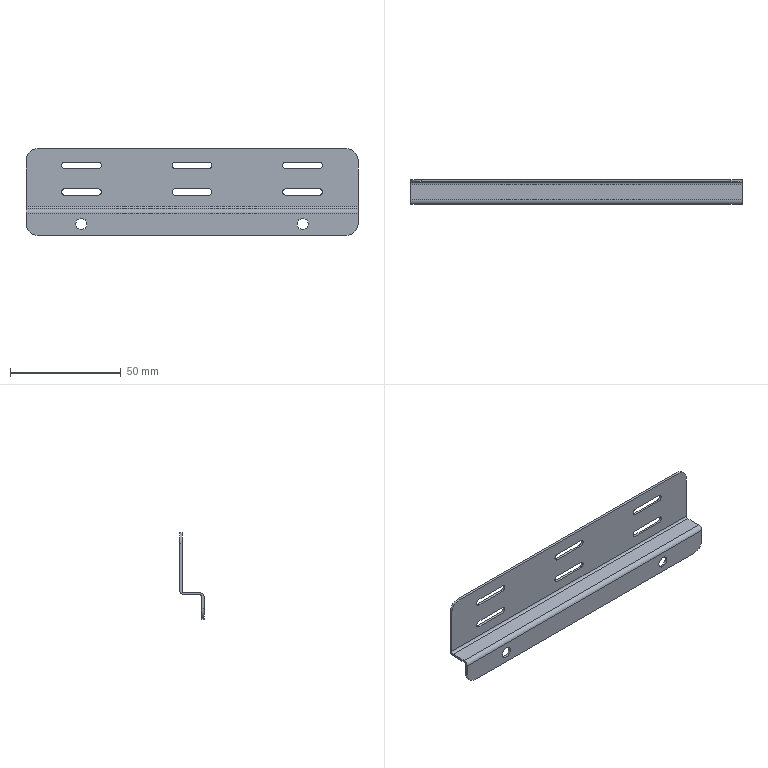Part | SolidWorks | features BaseBody 1 | 1 solid | 46 faces | box 150 x 11 x 39 mm | volume 6784 mm3 | cylinder 24 | plane 22 | commonest cylinder face diameters 3 x12 5 x4 10 x4 2 x2 4 x2
STEP:
#1=CARTESIAN_POINT('',(-50.,-11.,-23.));
#2=VERTEX_POINT('',#1);
#3=CARTESIAN_POINT('',(-50.,-11.,-18.));
#4=VERTEX_POINT('',#3);
#5=CARTESIAN_POINT('',(-50.,-11.,-20.5));
#6=DIRECTION('',(0.,1.,0.));
#7=DIRECTION('',(0.,0.,1.));
#8=AXIS2_PLACEMENT_3D('',#5,#6,#7);
#9=CIRCLE('',#8,2.5);
#10=EDGE_CURVE('',#2,#4,#9,.T.);
#11=ORIENTED_EDGE('',*,*,#10,.F.);
#12=CARTESIAN_POINT('',(-50.,-10.,-23.));
#13=VERTEX_POINT('',#12);
#14=CARTESIAN_POINT('',(-50.,-10.,-23.));
#15=DIRECTION('',(0.,1.,0.));
#16=VECTOR('',#15,1000.);
#17=LINE('',#14,#16);
#18=EDGE_CURVE('',#2,#13,#17,.T.);
#19=ORIENTED_EDGE('',*,*,#18,.T.);
#20=CARTESIAN_POINT('',(-50.,-10.,-18.));
#21=VERTEX_POINT('',#20);
#22=CARTESIAN_POINT('',(-50.,-10.,-20.5));
#23=DIRECTION('',(0.,1.,0.));
#24=DIRECTION('',(0.,0.,1.));
#25=AXIS2_PLACEMENT_3D('',#22,#23,#24);
#26=CIRCLE('',#25,2.5);
#27=EDGE_CURVE('',#13,#21,#26,.T.);
#28=ORIENTED_EDGE('',*,*,#27,.T.);
#29=CARTESIAN_POINT('',(-50.,-10.,-18.));
#30=DIRECTION('',(0.,1.,0.));
#31=VECTOR('',#30,1000.);
#32=LINE('',#29,#31);
#33=EDGE_CURVE('',#4,#21,#32,.T.);
#34=ORIENTED_EDGE('',*,*,#33,.F.);
#35=EDGE_LOOP('',(#11,#19,#28,#34));
#36=FACE_OUTER_BOUND('',#35,.T.);
#37=CARTESIAN_POINT('',(-50.,-10.,-20.5));
#38=DIRECTION('',(0.,1.,0.));
#39=DIRECTION('',(0.,0.,1.));
#40=AXIS2_PLACEMENT_3D('',#37,#38,#39);
#41=CYLINDRICAL_SURFACE('',#40,2.5);
#42=ADVANCED_FACE('',(#36),#41,.F.);
#43=CARTESIAN_POINT('',(50.,-11.,-23.));
#44=VERTEX_POINT('',#43);
#45=CARTESIAN_POINT('',(50.,-11.,-18.));
#46=VERTEX_POINT('',#45);
#47=CARTESIAN_POINT('',(50.,-11.,-20.5));
#48=DIRECTION('',(0.,1.,0.));
#49=DIRECTION('',(0.,0.,1.));
#50=AXIS2_PLACEMENT_3D('',#47,#48,#49);
#51=CIRCLE('',#50,2.5);
#52=EDGE_CURVE('',#44,#46,#51,.T.);
#53=ORIENTED_EDGE('',*,*,#52,.F.);
#54=CARTESIAN_POINT('',(50.,-10.,-23.));
#55=VERTEX_POINT('',#54);
#56=CARTESIAN_POINT('',(50.,-10.,-23.));
#57=DIRECTION('',(0.,1.,0.));
#58=VECTOR('',#57,1000.);
#59=LINE('',#56,#58);
#60=EDGE_CURVE('',#44,#55,#59,.T.);
#61=ORIENTED_EDGE('',*,*,#60,.T.);
#62=CARTESIAN_POINT('',(50.,-10.,-18.));
#63=VERTEX_POINT('',#62);
#64=CARTESIAN_POINT('',(50.,-10.,-20.5));
#65=DIRECTION('',(0.,1.,0.));
#66=DIRECTION('',(0.,0.,1.));
#67=AXIS2_PLACEMENT_3D('',#64,#65,#66);
#68=CIRCLE('',#67,2.5);
#69=EDGE_CURVE('',#55,#63,#68,.T.);
#70=ORIENTED_EDGE('',*,*,#69,.T.);
#71=CARTESIAN_POINT('',(50.,-10.,-18.));
#72=DIRECTION('',(0.,1.,0.));
#73=VECTOR('',#72,1000.);
#74=LINE('',#71,#73);
#75=EDGE_CURVE('',#46,#63,#74,.T.);
#76=ORIENTED_EDGE('',*,*,#75,.F.);
#77=EDGE_LOOP('',(#53,#61,#70,#76));
#78=FACE_OUTER_BOUND('',#77,.T.);
#79=CARTESIAN_POINT('',(50.,-10.,-20.5));
#80=DIRECTION('',(0.,1.,0.));
#81=DIRECTION('',(0.,0.,1.));
#82=AXIS2_PLACEMENT_3D('',#79,#80,#81);
#83=CYLINDRICAL_SURFACE('',#82,2.5);
#84=ADVANCED_FACE('',(#78),#83,.F.);
#85=CARTESIAN_POINT('',(7.5,-1.,-4.5));
#86=VERTEX_POINT('',#85);
#87=CARTESIAN_POINT('',(-7.5,-1.,-4.5));
#88=VERTEX_POINT('',#87);
#89=CARTESIAN_POINT('',(-7.5,-1.,-4.5));
#90=DIRECTION('',(-1.,0.,0.));
#91=VECTOR('',#90,1000.);
#92=LINE('',#89,#91);
#93=EDGE_CURVE('',#86,#88,#92,.T.);
#94=ORIENTED_EDGE('',*,*,#93,.T.);
#95=CARTESIAN_POINT('',(-7.5,0.,-4.5));
#96=VERTEX_POINT('',#95);
#97=CARTESIAN_POINT('',(-7.5,-11.001,-4.5));
#98=DIRECTION('',(0.,1.,0.));
#99=VECTOR('',#98,1000.);
#100=LINE('',#97,#99);
#101=EDGE_CURVE('',#88,#96,#100,.T.);
#102=ORIENTED_EDGE('',*,*,#101,.T.);
#103=CARTESIAN_POINT('',(7.5,0.,-4.5));
#104=VERTEX_POINT('',#103);
#105=CARTESIAN_POINT('',(-7.5,0.,-4.5));
#106=DIRECTION('',(1.,0.,0.));
#107=VECTOR('',#106,1000.);
#108=LINE('',#105,#107);
#109=EDGE_CURVE('',#96,#104,#108,.T.);
#110=ORIENTED_EDGE('',*,*,#109,.T.);
#111=CARTESIAN_POINT('',(7.5,-11.001,-4.5));
#112=DIRECTION('',(0.,1.,0.));
#113=VECTOR('',#112,1000.);
#114=LINE('',#111,#113);
#115=EDGE_CURVE('',#86,#104,#114,.T.);
#116=ORIENTED_EDGE('',*,*,#115,.F.);
#117=EDGE_LOOP('',(#94,#102,#110,#116));
#118=FACE_OUTER_BOUND('',#117,.T.);
#119=CARTESIAN_POINT('',(-7.5,-11.001,-4.5));
#120=DIRECTION('',(0.,0.,1.));
#121=DIRECTION('',(1.,0.,0.));
#122=AXIS2_PLACEMENT_3D('',#119,#120,#121);
#123=PLANE('',#122);
#124=ADVANCED_FACE('',(#118),#123,.F.);
#125=CARTESIAN_POINT('',(7.5,-1.,-7.5));
#126=VERTEX_POINT('',#125);
#127=CARTESIAN_POINT('',(7.5,-1.,-6.));
#128=DIRECTION('',(0.,-1.,0.));
#129=DIRECTION('',(0.,0.,1.));
#130=AXIS2_PLACEMENT_3D('',#127,#128,#129);
#131=CIRCLE('',#130,1.5);
#132=EDGE_CURVE('',#126,#86,#131,.T.);
#133=ORIENTED_EDGE('',*,*,#132,.T.);
#134=ORIENTED_EDGE('',*,*,#115,.T.);
#135=CARTESIAN_POINT('',(7.5,0.,-7.5));
#136=VERTEX_POINT('',#135);
#137=CARTESIAN_POINT('',(7.5,0.,-6.));
#138=DIRECTION('',(0.,1.,0.));
#139=DIRECTION('',(0.,0.,1.));
#140=AXIS2_PLACEMENT_3D('',#137,#138,#139);
#141=CIRCLE('',#140,1.5);
#142=EDGE_CURVE('',#104,#136,#141,.T.);
#143=ORIENTED_EDGE('',*,*,#142,.T.);
#144=CARTESIAN_POINT('',(7.5,-11.001,-7.5));
#145=DIRECTION('',(0.,1.,0.));
#146=VECTOR('',#145,1000.);
#147=LINE('',#144,#146);
#148=EDGE_CURVE('',#126,#136,#147,.T.);
#149=ORIENTED_EDGE('',*,*,#148,.F.);
#150=EDGE_LOOP('',(#133,#134,#143,#149));
#151=FACE_OUTER_BOUND('',#150,.T.);
#152=CARTESIAN_POINT('',(7.5,-11.001,-6.));
#153=DIRECTION('',(0.,1.,0.));
#154=DIRECTION('',(0.,0.,1.));
#155=AXIS2_PLACEMENT_3D('',#152,#153,#154);
#156=CYLINDRICAL_SURFACE('',#155,1.5);
#157=ADVANCED_FACE('',(#151),#156,.F.);
#158=CARTESIAN_POINT('',(-7.5,-1.,-7.5));
#159=VERTEX_POINT('',#158);
#160=CARTESIAN_POINT('',(-7.5,-1.,-7.5));
#161=DIRECTION('',(1.,0.,0.));
#162=VECTOR('',#161,1000.);
#163=LINE('',#160,#162);
#164=EDGE_CURVE('',#159,#126,#163,.T.);
#165=ORIENTED_EDGE('',*,*,#164,.T.);
#166=ORIENTED_EDGE('',*,*,#148,.T.);
#167=CARTESIAN_POINT('',(-7.5,0.,-7.5));
#168=VERTEX_POINT('',#167);
#169=CARTESIAN_POINT('',(-7.5,0.,-7.5));
#170=DIRECTION('',(-1.,0.,0.));
#171=VECTOR('',#170,1000.);
#172=LINE('',#169,#171);
#173=EDGE_CURVE('',#136,#168,#172,.T.);
#174=ORIENTED_EDGE('',*,*,#173,.T.);
#175=CARTESIAN_POINT('',(-7.5,-11.001,-7.5));
#176=DIRECTION('',(0.,1.,0.));
#177=VECTOR('',#176,1000.);
#178=LINE('',#175,#177);
#179=EDGE_CURVE('',#159,#168,#178,.T.);
#180=ORIENTED_EDGE('',*,*,#179,.F.);
#181=EDGE_LOOP('',(#165,#166,#174,#180));
#182=FACE_OUTER_BOUND('',#181,.T.);
#183=CARTESIAN_POINT('',(-7.5,-11.001,-7.5));
#184=DIRECTION('',(0.,0.,-1.));
#185=DIRECTION('',(-1.,0.,0.));
#186=AXIS2_PLACEMENT_3D('',#183,#184,#185);
#187=PLANE('',#186);
#188=ADVANCED_FACE('',(#182),#187,.F.);
#189=CARTESIAN_POINT('',(-7.5,-1.,-6.));
#190=DIRECTION('',(0.,-1.,0.));
#191=DIRECTION('',(0.,0.,1.));
#192=AXIS2_PLACEMENT_3D('',#189,#190,#191);
#193=CIRCLE('',#192,1.5);
#194=EDGE_CURVE('',#88,#159,#193,.T.);
#195=ORIENTED_EDGE('',*,*,#194,.T.);
#196=ORIENTED_EDGE('',*,*,#179,.T.);
#197=CARTESIAN_POINT('',(-7.5,0.,-6.));
#198=DIRECTION('',(0.,1.,0.));
#199=DIRECTION('',(0.,0.,1.));
#200=AXIS2_PLACEMENT_3D('',#197,#198,#199);
#201=CIRCLE('',#200,1.5);
#202=EDGE_CURVE('',#168,#96,#201,.T.);
#203=ORIENTED_EDGE('',*,*,#202,.T.);
#204=ORIENTED_EDGE('',*,*,#101,.F.);
#205=EDGE_LOOP('',(#195,#196,#203,#204));
#206=FACE_OUTER_BOUND('',#205,.T.);
#207=CARTESIAN_POINT('',(-7.5,-11.001,-6.));
#208=DIRECTION('',(0.,1.,0.));
#209=DIRECTION('',(0.,0.,1.));
#210=AXIS2_PLACEMENT_3D('',#207,#208,#209);
#211=CYLINDRICAL_SURFACE('',#210,1.5);
#212=ADVANCED_FACE('',(#206),#211,.F.);
#213=CARTESIAN_POINT('',(7.5,-1.,7.5));
#214=VERTEX_POINT('',#213);
#215=CARTESIAN_POINT('',(-7.5,-1.,7.5));
#216=VERTEX_POINT('',#215);
#217=CARTESIAN_POINT('',(-7.5,-1.,7.5));
#218=DIRECTION('',(-1.,0.,0.));
#219=VECTOR('',#218,1000.);
#220=LINE('',#217,#219);
#221=EDGE_CURVE('',#214,#216,#220,.T.);
#222=ORIENTED_EDGE('',*,*,#221,.T.);
#223=CARTESIAN_POINT('',(-7.5,0.,7.5));
#224=VERTEX_POINT('',#223);
#225=CARTESIAN_POINT('',(-7.5,-11.001,7.5));
#226=DIRECTION('',(0.,1.,0.));
#227=VECTOR('',#226,1000.);
#228=LINE('',#225,#227);
#229=EDGE_CURVE('',#216,#224,#228,.T.);
#230=ORIENTED_EDGE('',*,*,#229,.T.);
#231=CARTESIAN_POINT('',(7.5,0.,7.5));
#232=VERTEX_POINT('',#231);
#233=CARTESIAN_POINT('',(-7.5,0.,7.5));
#234=DIRECTION('',(1.,0.,0.));
#235=VECTOR('',#234,1000.);
#236=LINE('',#233,#235);
#237=EDGE_CURVE('',#224,#232,#236,.T.);
#238=ORIENTED_EDGE('',*,*,#237,.T.);
#239=CARTESIAN_POINT('',(7.5,-11.001,7.5));
#240=DIRECTION('',(0.,1.,0.));
#241=VECTOR('',#240,1000.);
#242=LINE('',#239,#241);
#243=EDGE_CURVE('',#214,#232,#242,.T.);
#244=ORIENTED_EDGE('',*,*,#243,.F.);
#245=EDGE_LOOP('',(#222,#230,#238,#244));
#246=FACE_OUTER_BOUND('',#245,.T.);
#247=CARTESIAN_POINT('',(-7.5,-11.001,7.5));
#248=DIRECTION('',(0.,0.,1.));
#249=DIRECTION('',(1.,0.,0.));
#250=AXIS2_PLACEMENT_3D('',#247,#248,#249);
#251=PLANE('',#250);
#252=ADVANCED_FACE('',(#246),#251,.F.);
#253=CARTESIAN_POINT('',(7.5,-1.,4.5));
#254=VERTEX_POINT('',#253);
#255=CARTESIAN_POINT('',(7.5,-1.,6.));
#256=DIRECTION('',(0.,-1.,0.));
#257=DIRECTION('',(0.,0.,1.));
#258=AXIS2_PLACEMENT_3D('',#255,#256,#257);
#259=CIRCLE('',#258,1.5);
#260=EDGE_CURVE('',#254,#214,#259,.T.);
#261=ORIENTED_EDGE('',*,*,#260,.T.);
#262=ORIENTED_EDGE('',*,*,#243,.T.);
#263=CARTESIAN_POINT('',(7.5,0.,4.5));
#264=VERTEX_POINT('',#263);
#265=CARTESIAN_POINT('',(7.5,0.,6.));
#266=DIRECTION('',(0.,1.,0.));
#267=DIRECTION('',(0.,0.,1.));
#268=AXIS2_PLACEMENT_3D('',#265,#266,#267);
#269=CIRCLE('',#268,1.5);
#270=EDGE_CURVE('',#232,#264,#269,.T.);
#271=ORIENTED_EDGE('',*,*,#270,.T.);
#272=CARTESIAN_POINT('',(7.5,-11.001,4.5));
#273=DIRECTION('',(0.,1.,0.));
#274=VECTOR('',#273,1000.);
#275=LINE('',#272,#274);
#276=EDGE_CURVE('',#254,#264,#275,.T.);
#277=ORIENTED_EDGE('',*,*,#276,.F.);
#278=EDGE_LOOP('',(#261,#262,#271,#277));
#279=FACE_OUTER_BOUND('',#278,.T.);
#280=CARTESIAN_POINT('',(7.5,-11.001,6.));
#281=DIRECTION('',(0.,1.,0.));
#282=DIRECTION('',(0.,0.,1.));
#283=AXIS2_PLACEMENT_3D('',#280,#281,#282);
#284=CYLINDRICAL_SURFACE('',#283,1.5);
#285=ADVANCED_FACE('',(#279),#284,.F.);
#286=CARTESIAN_POINT('',(-7.5,-1.,4.5));
#287=VERTEX_POINT('',#286);
#288=CARTESIAN_POINT('',(-7.5,-1.,4.5));
#289=DIRECTION('',(1.,0.,0.));
#290=VECTOR('',#289,1000.);
#291=LINE('',#288,#290);
#292=EDGE_CURVE('',#287,#254,#291,.T.);
#293=ORIENTED_EDGE('',*,*,#292,.T.);
#294=ORIENTED_EDGE('',*,*,#276,.T.);
#295=CARTESIAN_POINT('',(-7.5,0.,4.5));
#296=VERTEX_POINT('',#295);
#297=CARTESIAN_POINT('',(-7.5,0.,4.5));
#298=DIRECTION('',(-1.,0.,0.));
#299=VECTOR('',#298,1000.);
#300=LINE('',#297,#299);
#301=EDGE_CURVE('',#264,#296,#300,.T.);
#302=ORIENTED_EDGE('',*,*,#301,.T.);
#303=CARTESIAN_POINT('',(-7.5,-11.001,4.5));
#304=DIRECTION('',(0.,1.,0.));
#305=VECTOR('',#304,1000.);
#306=LINE('',#303,#305);
#307=EDGE_CURVE('',#287,#296,#306,.T.);
#308=ORIENTED_EDGE('',*,*,#307,.F.);
#309=EDGE_LOOP('',(#293,#294,#302,#308));
#310=FACE_OUTER_BOUND('',#309,.T.);
#311=CARTESIAN_POINT('',(-7.5,-11.001,4.5));
#312=DIRECTION('',(0.,0.,-1.));
#313=DIRECTION('',(0.,-1.,0.));
#314=AXIS2_PLACEMENT_3D('',#311,#312,#313);
#315=PLANE('',#314);
#316=ADVANCED_FACE('',(#310),#315,.F.);
#317=CARTESIAN_POINT('',(-7.5,-1.,6.));
#318=DIRECTION('',(0.,-1.,0.));
#319=DIRECTION('',(0.,0.,1.));
#320=AXIS2_PLACEMENT_3D('',#317,#318,#319);
#321=CIRCLE('',#320,1.5);
#322=EDGE_CURVE('',#216,#287,#321,.T.);
#323=ORIENTED_EDGE('',*,*,#322,.T.);
#324=ORIENTED_EDGE('',*,*,#307,.T.);
#325=CARTESIAN_POINT('',(-7.5,0.,6.));
#326=DIRECTION('',(0.,1.,0.));
#327=DIRECTION('',(0.,0.,1.));
#328=AXIS2_PLACEMENT_3D('',#325,#326,#327);
#329=CIRCLE('',#328,1.5);
#330=EDGE_CURVE('',#296,#224,#329,.T.);
#331=ORIENTED_EDGE('',*,*,#330,.T.);
#332=ORIENTED_EDGE('',*,*,#229,.F.);
#333=EDGE_LOOP('',(#323,#324,#331,#332));
#334=FACE_OUTER_BOUND('',#333,.T.);
#335=CARTESIAN_POINT('',(-7.5,-11.001,6.));
#336=DIRECTION('',(0.,1.,0.));
#337=DIRECTION('',(0.,0.,1.));
#338=AXIS2_PLACEMENT_3D('',#335,#336,#337);
#339=CYLINDRICAL_SURFACE('',#338,1.5);
#340=ADVANCED_FACE('',(#334),#339,.F.);
#341=CARTESIAN_POINT('',(-42.5,-1.,7.5));
#342=VERTEX_POINT('',#341);
#343=CARTESIAN_POINT('',(-57.5,-1.,7.5));
#344=VERTEX_POINT('',#343);
#345=CARTESIAN_POINT('',(-57.5,-1.,7.5));
#346=DIRECTION('',(-1.,0.,0.));
#347=VECTOR('',#346,1000.);
#348=LINE('',#345,#347);
#349=EDGE_CURVE('',#342,#344,#348,.T.);
#350=ORIENTED_EDGE('',*,*,#349,.T.);
#351=CARTESIAN_POINT('',(-57.5,0.,7.5));
#352=VERTEX_POINT('',#351);
#353=CARTESIAN_POINT('',(-57.5,-11.001,7.5));
#354=DIRECTION('',(0.,1.,0.));
#355=VECTOR('',#354,1000.);
#356=LINE('',#353,#355);
#357=EDGE_CURVE('',#344,#352,#356,.T.);
#358=ORIENTED_EDGE('',*,*,#357,.T.);
#359=CARTESIAN_POINT('',(-42.5,0.,7.5));
#360=VERTEX_POINT('',#359);
#361=CARTESIAN_POINT('',(-57.5,0.,7.5));
#362=DIRECTION('',(1.,0.,0.));
#363=VECTOR('',#362,1000.);
#364=LINE('',#361,#363);
#365=EDGE_CURVE('',#352,#360,#364,.T.);
#366=ORIENTED_EDGE('',*,*,#365,.T.);
#367=CARTESIAN_POINT('',(-42.5,-11.001,7.5));
#368=DIRECTION('',(0.,1.,0.));
#369=VECTOR('',#368,1000.);
#370=LINE('',#367,#369);
#371=EDGE_CURVE('',#342,#360,#370,.T.);
#372=ORIENTED_EDGE('',*,*,#371,.F.);
#373=EDGE_LOOP('',(#350,#358,#366,#372));
#374=FACE_OUTER_BOUND('',#373,.T.);
#375=CARTESIAN_POINT('',(-57.5,-11.001,7.5));
#376=DIRECTION('',(0.,0.,1.));
#377=DIRECTION('',(1.,0.,0.));
#378=AXIS2_PLACEMENT_3D('',#375,#376,#377);
#379=PLANE('',#378);
#380=ADVANCED_FACE('',(#374),#379,.F.);
#381=CARTESIAN_POINT('',(-42.5,-1.,4.5));
#382=VERTEX_POINT('',#381);
#383=CARTESIAN_POINT('',(-42.5,-1.,6.));
#384=DIRECTION('',(0.,-1.,0.));
#385=DIRECTION('',(0.,0.,1.));
#386=AXIS2_PLACEMENT_3D('',#383,#384,#385);
#387=CIRCLE('',#386,1.5);
#388=EDGE_CURVE('',#382,#342,#387,.T.);
#389=ORIENTED_EDGE('',*,*,#388,.T.);
#390=ORIENTED_EDGE('',*,*,#371,.T.);
#391=CARTESIAN_POINT('',(-42.5,0.,4.5));
#392=VERTEX_POINT('',#391);
#393=CARTESIAN_POINT('',(-42.5,0.,6.));
#394=DIRECTION('',(0.,1.,0.));
#395=DIRECTION('',(0.,0.,1.));
#396=AXIS2_PLACEMENT_3D('',#393,#394,#395);
#397=CIRCLE('',#396,1.5);
#398=EDGE_CURVE('',#360,#392,#397,.T.);
#399=ORIENTED_EDGE('',*,*,#398,.T.);
#400=CARTESIAN_POINT('',(-42.5,-11.001,4.5));
#401=DIRECTION('',(0.,1.,0.));
#402=VECTOR('',#401,1000.);
#403=LINE('',#400,#402);
#404=EDGE_CURVE('',#382,#392,#403,.T.);
#405=ORIENTED_EDGE('',*,*,#404,.F.);
#406=EDGE_LOOP('',(#389,#390,#399,#405));
#407=FACE_OUTER_BOUND('',#406,.T.);
#408=CARTESIAN_POINT('',(-42.5,-11.001,6.));
#409=DIRECTION('',(0.,1.,0.));
#410=DIRECTION('',(0.,0.,1.));
#411=AXIS2_PLACEMENT_3D('',#408,#409,#410);
#412=CYLINDRICAL_SURFACE('',#411,1.5);
#413=ADVANCED_FACE('',(#407),#412,.F.);
#414=CARTESIAN_POINT('',(-57.5,-1.,4.5));
#415=VERTEX_POINT('',#414);
#416=CARTESIAN_POINT('',(-57.5,-1.,4.5));
#417=DIRECTION('',(1.,0.,0.));
#418=VECTOR('',#417,1000.);
#419=LINE('',#416,#418);
#420=EDGE_CURVE('',#415,#382,#419,.T.);
#421=ORIENTED_EDGE('',*,*,#420,.T.);
#422=ORIENTED_EDGE('',*,*,#404,.T.);
#423=CARTESIAN_POINT('',(-57.5,0.,4.5));
#424=VERTEX_POINT('',#423);
#425=CARTESIAN_POINT('',(-57.5,0.,4.5));
#426=DIRECTION('',(-1.,0.,0.));
#427=VECTOR('',#426,1000.);
#428=LINE('',#425,#427);
#429=EDGE_CURVE('',#392,#424,#428,.T.);
#430=ORIENTED_EDGE('',*,*,#429,.T.);
#431=CARTESIAN_POINT('',(-57.5,-11.001,4.5));
#432=DIRECTION('',(0.,1.,0.));
#433=VECTOR('',#432,1000.);
#434=LINE('',#431,#433);
#435=EDGE_CURVE('',#415,#424,#434,.T.);
#436=ORIENTED_EDGE('',*,*,#435,.F.);
#437=EDGE_LOOP('',(#421,#422,#430,#436));
#438=FACE_OUTER_BOUND('',#437,.T.);
#439=CARTESIAN_POINT('',(-57.5,-11.001,4.5));
#440=DIRECTION('',(0.,0.,-1.));
#441=DIRECTION('',(0.,-1.,0.));
#442=AXIS2_PLACEMENT_3D('',#439,#440,#441);
#443=PLANE('',#442);
#444=ADVANCED_FACE('',(#438),#443,.F.);
#445=CARTESIAN_POINT('',(-57.5,-1.,6.));
#446=DIRECTION('',(0.,-1.,0.));
#447=DIRECTION('',(0.,0.,1.));
#448=AXIS2_PLACEMENT_3D('',#445,#446,#447);
#449=CIRCLE('',#448,1.5);
#450=EDGE_CURVE('',#344,#415,#449,.T.);
#451=ORIENTED_EDGE('',*,*,#450,.T.);
#452=ORIENTED_EDGE('',*,*,#435,.T.);
#453=CARTESIAN_POINT('',(-57.5,0.,6.));
#454=DIRECTION('',(0.,1.,0.));
#455=DIRECTION('',(0.,0.,1.));
#456=AXIS2_PLACEMENT_3D('',#453,#454,#455);
#457=CIRCLE('',#456,1.5);
#458=EDGE_CURVE('',#424,#352,#457,.T.);
#459=ORIENTED_EDGE('',*,*,#458,.T.);
#460=ORIENTED_EDGE('',*,*,#357,.F.);
#461=EDGE_LOOP('',(#451,#452,#459,#460));
#462=FACE_OUTER_BOUND('',#461,.T.);
#463=CARTESIAN_POINT('',(-57.5,-11.001,6.));
#464=DIRECTION('',(0.,1.,0.));
#465=DIRECTION('',(0.,0.,1.));
#466=AXIS2_PLACEMENT_3D('',#463,#464,#465);
#467=CYLINDRICAL_SURFACE('',#466,1.5);
#468=ADVANCED_FACE('',(#462),#467,.F.);
#469=CARTESIAN_POINT('',(-42.5,-1.,-4.5));
#470=VERTEX_POINT('',#469);
#471=CARTESIAN_POINT('',(-57.5,-1.,-4.5));
#472=VERTEX_POINT('',#471);
#473=CARTESIAN_POINT('',(-57.5,-1.,-4.5));
#474=DIRECTION('',(-1.,0.,0.));
#475=VECTOR('',#474,1000.);
#476=LINE('',#473,#475);
#477=EDGE_CURVE('',#470,#472,#476,.T.);
#478=ORIENTED_EDGE('',*,*,#477,.T.);
#479=CARTESIAN_POINT('',(-57.5,0.,-4.5));
#480=VERTEX_POINT('',#479);
#481=CARTESIAN_POINT('',(-57.5,-11.001,-4.5));
#482=DIRECTION('',(0.,1.,0.));
#483=VECTOR('',#482,1000.);
#484=LINE('',#481,#483);
#485=EDGE_CURVE('',#472,#480,#484,.T.);
#486=ORIENTED_EDGE('',*,*,#485,.T.);
#487=CARTESIAN_POINT('',(-42.5,0.,-4.5));
#488=VERTEX_POINT('',#487);
#489=CARTESIAN_POINT('',(-57.5,0.,-4.5));
#490=DIRECTION('',(1.,0.,0.));
#491=VECTOR('',#490,1000.);
#492=LINE('',#489,#491);
#493=EDGE_CURVE('',#480,#488,#492,.T.);
#494=ORIENTED_EDGE('',*,*,#493,.T.);
#495=CARTESIAN_POINT('',(-42.5,-11.001,-4.5));
#496=DIRECTION('',(0.,1.,0.));
#497=VECTOR('',#496,1000.);
#498=LINE('',#495,#497);
#499=EDGE_CURVE('',#470,#488,#498,.T.);
#500=ORIENTED_EDGE('',*,*,#499,.F.);
#501=EDGE_LOOP('',(#478,#486,#494,#500));
#502=FACE_OUTER_BOUND('',#501,.T.);
#503=CARTESIAN_POINT('',(-57.5,-11.001,-4.5));
#504=DIRECTION('',(0.,0.,1.));
#505=DIRECTION('',(1.,0.,0.));
#506=AXIS2_PLACEMENT_3D('',#503,#504,#505);
#507=PLANE('',#506);
#508=ADVANCED_FACE('',(#502),#507,.F.);
#509=CARTESIAN_POINT('',(-42.5,-1.,-7.5));
#510=VERTEX_POINT('',#509);
#511=CARTESIAN_POINT('',(-42.5,-1.,-6.));
#512=DIRECTION('',(0.,-1.,0.));
#513=DIRECTION('',(0.,0.,1.));
#514=AXIS2_PLACEMENT_3D('',#511,#512,#513);
#515=CIRCLE('',#514,1.5);
#516=EDGE_CURVE('',#510,#470,#515,.T.);
#517=ORIENTED_EDGE('',*,*,#516,.T.);
#518=ORIENTED_EDGE('',*,*,#499,.T.);
#519=CARTESIAN_POINT('',(-42.5,0.,-7.5));
#520=VERTEX_POINT('',#519);
#521=CARTESIAN_POINT('',(-42.5,0.,-6.));
#522=DIRECTION('',(0.,1.,0.));
#523=DIRECTION('',(0.,0.,1.));
#524=AXIS2_PLACEMENT_3D('',#521,#522,#523);
#525=CIRCLE('',#524,1.5);
#526=EDGE_CURVE('',#488,#520,#525,.T.);
#527=ORIENTED_EDGE('',*,*,#526,.T.);
#528=CARTESIAN_POINT('',(-42.5,-11.001,-7.5));
#529=DIRECTION('',(0.,1.,0.));
#530=VECTOR('',#529,1000.);
#531=LINE('',#528,#530);
#532=EDGE_CURVE('',#510,#520,#531,.T.);
#533=ORIENTED_EDGE('',*,*,#532,.F.);
#534=EDGE_LOOP('',(#517,#518,#527,#533));
#535=FACE_OUTER_BOUND('',#534,.T.);
#536=CARTESIAN_POINT('',(-42.5,-11.001,-6.));
#537=DIRECTION('',(0.,1.,0.));
#538=DIRECTION('',(0.,0.,1.));
#539=AXIS2_PLACEMENT_3D('',#536,#537,#538);
#540=CYLINDRICAL_SURFACE('',#539,1.5);
#541=ADVANCED_FACE('',(#535),#540,.F.);
#542=CARTESIAN_POINT('',(-57.5,-1.,-7.5));
#543=VERTEX_POINT('',#542);
#544=CARTESIAN_POINT('',(-57.5,-1.,-7.5));
#545=DIRECTION('',(1.,0.,0.));
#546=VECTOR('',#545,1000.);
#547=LINE('',#544,#546);
#548=EDGE_CURVE('',#543,#510,#547,.T.);
#549=ORIENTED_EDGE('',*,*,#548,.T.);
#550=ORIENTED_EDGE('',*,*,#532,.T.);
#551=CARTESIAN_POINT('',(-57.5,0.,-7.5));
#552=VERTEX_POINT('',#551);
#553=CARTESIAN_POINT('',(-57.5,0.,-7.5));
#554=DIRECTION('',(-1.,0.,0.));
#555=VECTOR('',#554,1000.);
#556=LINE('',#553,#555);
#557=EDGE_CURVE('',#520,#552,#556,.T.);
#558=ORIENTED_EDGE('',*,*,#557,.T.);
#559=CARTESIAN_POINT('',(-57.5,-11.001,-7.5));
#560=DIRECTION('',(0.,1.,0.));
#561=VECTOR('',#560,1000.);
#562=LINE('',#559,#561);
#563=EDGE_CURVE('',#543,#552,#562,.T.);
#564=ORIENTED_EDGE('',*,*,#563,.F.);
#565=EDGE_LOOP('',(#549,#550,#558,#564));
#566=FACE_OUTER_BOUND('',#565,.T.);
#567=CARTESIAN_POINT('',(-57.5,-11.001,-7.5));
#568=DIRECTION('',(0.,0.,-1.));
#569=DIRECTION('',(-1.,0.,0.));
#570=AXIS2_PLACEMENT_3D('',#567,#568,#569);
#571=PLANE('',#570);
#572=ADVANCED_FACE('',(#566),#571,.F.);
#573=CARTESIAN_POINT('',(-57.5,-1.,-6.));
#574=DIRECTION('',(0.,-1.,0.));
#575=DIRECTION('',(0.,0.,1.));
#576=AXIS2_PLACEMENT_3D('',#573,#574,#575);
#577=CIRCLE('',#576,1.5);
#578=EDGE_CURVE('',#472,#543,#577,.T.);
#579=ORIENTED_EDGE('',*,*,#578,.T.);
#580=ORIENTED_EDGE('',*,*,#563,.T.);
#581=CARTESIAN_POINT('',(-57.5,0.,-6.));
#582=DIRECTION('',(0.,1.,0.));
#583=DIRECTION('',(0.,0.,1.));
#584=AXIS2_PLACEMENT_3D('',#581,#582,#583);
#585=CIRCLE('',#584,1.5);
#586=EDGE_CURVE('',#552,#480,#585,.T.);
#587=ORIENTED_EDGE('',*,*,#586,.T.);
#588=ORIENTED_EDGE('',*,*,#485,.F.);
#589=EDGE_LOOP('',(#579,#580,#587,#588));
#590=FACE_OUTER_BOUND('',#589,.T.);
#591=CARTESIAN_POINT('',(-57.5,-11.001,-6.));
#592=DIRECTION('',(0.,1.,0.));
#593=DIRECTION('',(0.,0.,1.));
#594=AXIS2_PLACEMENT_3D('',#591,#592,#593);
#595=CYLINDRICAL_SURFACE('',#594,1.5);
#596=ADVANCED_FACE('',(#590),#595,.F.);
#597=CARTESIAN_POINT('',(-75.,-11.,-20.5));
#598=VERTEX_POINT('',#597);
#599=CARTESIAN_POINT('',(-70.,-11.,-25.5));
#600=VERTEX_POINT('',#599);
#601=CARTESIAN_POINT('',(-70.,-11.,-20.5));
#602=DIRECTION('',(0.,-1.,0.));
#603=DIRECTION('',(0.,0.,1.));
#604=AXIS2_PLACEMENT_3D('',#601,#602,#603);
#605=CIRCLE('',#604,5.);
#606=EDGE_CURVE('',#598,#600,#605,.T.);
#607=ORIENTED_EDGE('',*,*,#606,.F.);
#608=CARTESIAN_POINT('',(-75.,-10.,-20.5));
#609=VERTEX_POINT('',#608);
#610=CARTESIAN_POINT('',(-75.,-11.,-20.5));
#611=DIRECTION('',(0.,-1.,0.));
#612=VECTOR('',#611,1000.);
#613=LINE('',#610,#612);
#614=EDGE_CURVE('',#609,#598,#613,.T.);
#615=ORIENTED_EDGE('',*,*,#614,.F.);
#616=CARTESIAN_POINT('',(-70.,-10.,-25.5));
#617=VERTEX_POINT('',#616);
#618=CARTESIAN_POINT('',(-70.,-10.,-20.5));
#619=DIRECTION('',(0.,1.,0.));
#620=DIRECTION('',(0.,0.,1.));
#621=AXIS2_PLACEMENT_3D('',#618,#619,#620);
#622=CIRCLE('',#621,5.);
#623=EDGE_CURVE('',#617,#609,#622,.T.);
#624=ORIENTED_EDGE('',*,*,#623,.F.);
#625=CARTESIAN_POINT('',(-70.,-11.,-25.5));
#626=DIRECTION('',(0.,1.,0.));
#627=VECTOR('',#626,1000.);
#628=LINE('',#625,#627);
#629=EDGE_CURVE('',#600,#617,#628,.T.);
#630=ORIENTED_EDGE('',*,*,#629,.F.);
#631=EDGE_LOOP('',(#607,#615,#624,#630));
#632=FACE_OUTER_BOUND('',#631,.T.);
#633=CARTESIAN_POINT('',(-70.,-11.,-20.5));
#634=DIRECTION('',(0.,1.,0.));
#635=DIRECTION('',(0.,0.,1.));
#636=AXIS2_PLACEMENT_3D('',#633,#634,#635);
#637=CYLINDRICAL_SURFACE('',#636,5.);
#638=ADVANCED_FACE('',(#632),#637,.T.);
#639=CARTESIAN_POINT('',(70.,-11.,-25.5));
#640=VERTEX_POINT('',#639);
#641=CARTESIAN_POINT('',(75.,-11.,-20.5));
#642=VERTEX_POINT('',#641);
#643=CARTESIAN_POINT('',(70.,-11.,-20.5));
#644=DIRECTION('',(0.,-1.,0.));
#645=DIRECTION('',(0.,0.,1.));
#646=AXIS2_PLACEMENT_3D('',#643,#644,#645);
#647=CIRCLE('',#646,5.);
#648=EDGE_CURVE('',#640,#642,#647,.T.);
#649=ORIENTED_EDGE('',*,*,#648,.F.);
#650=CARTESIAN_POINT('',(70.,-10.,-25.5));
#651=VERTEX_POINT('',#650);
#652=CARTESIAN_POINT('',(70.,-11.,-25.5));
#653=DIRECTION('',(0.,-1.,0.));
#654=VECTOR('',#653,1000.);
#655=LINE('',#652,#654);
#656=EDGE_CURVE('',#651,#640,#655,.T.);
#657=ORIENTED_EDGE('',*,*,#656,.F.);
#658=CARTESIAN_POINT('',(75.,-10.,-20.5));
#659=VERTEX_POINT('',#658);
#660=CARTESIAN_POINT('',(70.,-10.,-20.5));
#661=DIRECTION('',(0.,1.,0.));
#662=DIRECTION('',(0.,0.,1.));
#663=AXIS2_PLACEMENT_3D('',#660,#661,#662);
#664=CIRCLE('',#663,5.);
#665=EDGE_CURVE('',#659,#651,#664,.T.);
#666=ORIENTED_EDGE('',*,*,#665,.F.);
#667=CARTESIAN_POINT('',(75.,-11.,-20.5));
#668=DIRECTION('',(0.,1.,0.));
#669=VECTOR('',#668,1000.);
#670=LINE('',#667,#669);
#671=EDGE_CURVE('',#642,#659,#670,.T.);
#672=ORIENTED_EDGE('',*,*,#671,.F.);
#673=EDGE_LOOP('',(#649,#657,#666,#672));
#674=FACE_OUTER_BOUND('',#673,.T.);
#675=CARTESIAN_POINT('',(70.,-11.,-20.5));
#676=DIRECTION('',(0.,1.,0.));
#677=DIRECTION('',(0.,0.,1.));
#678=AXIS2_PLACEMENT_3D('',#675,#676,#677);
#679=CYLINDRICAL_SURFACE('',#678,5.);
#680=ADVANCED_FACE('',(#674),#679,.T.);
#681=CARTESIAN_POINT('',(75.,-1.,8.5));
#682=VERTEX_POINT('',#681);
#683=CARTESIAN_POINT('',(70.,-1.,13.5));
#684=VERTEX_POINT('',#683);
#685=CARTESIAN_POINT('',(70.,-1.,8.5));
#686=DIRECTION('',(0.,-1.,0.));
#687=DIRECTION('',(0.,0.,1.));
#688=AXIS2_PLACEMENT_3D('',#685,#686,#687);
#689=CIRCLE('',#688,5.);
#690=EDGE_CURVE('',#682,#684,#689,.T.);
#691=ORIENTED_EDGE('',*,*,#690,.F.);
#692=CARTESIAN_POINT('',(75.,0.,8.5));
#693=VERTEX_POINT('',#692);
#694=CARTESIAN_POINT('',(75.,-1.,8.5));
#695=DIRECTION('',(0.,-1.,0.));
#696=VECTOR('',#695,1000.);
#697=LINE('',#694,#696);
#698=EDGE_CURVE('',#693,#682,#697,.T.);
#699=ORIENTED_EDGE('',*,*,#698,.F.);
#700=CARTESIAN_POINT('',(70.,0.,13.5));
#701=VERTEX_POINT('',#700);
#702=CARTESIAN_POINT('',(70.,0.,8.5));
#703=DIRECTION('',(0.,1.,0.));
#704=DIRECTION('',(0.,0.,1.));
#705=AXIS2_PLACEMENT_3D('',#702,#703,#704);
#706=CIRCLE('',#705,5.);
#707=EDGE_CURVE('',#701,#693,#706,.T.);
#708=ORIENTED_EDGE('',*,*,#707,.F.);
#709=CARTESIAN_POINT('',(70.,-1.,13.5));
#710=DIRECTION('',(0.,1.,0.));
#711=VECTOR('',#710,1000.);
#712=LINE('',#709,#711);
#713=EDGE_CURVE('',#684,#701,#712,.T.);
#714=ORIENTED_EDGE('',*,*,#713,.F.);
#715=EDGE_LOOP('',(#691,#699,#708,#714));
#716=FACE_OUTER_BOUND('',#715,.T.);
#717=CARTESIAN_POINT('',(70.,-1.,8.5));
#718=DIRECTION('',(0.,1.,0.));
#719=DIRECTION('',(0.,0.,1.));
#720=AXIS2_PLACEMENT_3D('',#717,#718,#719);
#721=CYLINDRICAL_SURFACE('',#720,5.);
#722=ADVANCED_FACE('',(#716),#721,.T.);
#723=CARTESIAN_POINT('',(-70.,-1.,13.5));
#724=VERTEX_POINT('',#723);
#725=CARTESIAN_POINT('',(-75.,-1.,8.5));
#726=VERTEX_POINT('',#725);
#727=CARTESIAN_POINT('',(-70.,-1.,8.5));
#728=DIRECTION('',(0.,-1.,0.));
#729=DIRECTION('',(0.,0.,1.));
#730=AXIS2_PLACEMENT_3D('',#727,#728,#729);
#731=CIRCLE('',#730,5.);
#732=EDGE_CURVE('',#724,#726,#731,.T.);
#733=ORIENTED_EDGE('',*,*,#732,.F.);
#734=CARTESIAN_POINT('',(-70.,0.,13.5));
#735=VERTEX_POINT('',#734);
#736=CARTESIAN_POINT('',(-70.,-1.,13.5));
#737=DIRECTION('',(0.,-1.,0.));
#738=VECTOR('',#737,1000.);
#739=LINE('',#736,#738);
#740=EDGE_CURVE('',#735,#724,#739,.T.);
#741=ORIENTED_EDGE('',*,*,#740,.F.);
#742=CARTESIAN_POINT('',(-75.,0.,8.5));
#743=VERTEX_POINT('',#742);
#744=CARTESIAN_POINT('',(-70.,0.,8.5));
#745=DIRECTION('',(0.,1.,0.));
#746=DIRECTION('',(0.,0.,1.));
#747=AXIS2_PLACEMENT_3D('',#744,#745,#746);
#748=CIRCLE('',#747,5.);
#749=EDGE_CURVE('',#743,#735,#748,.T.);
#750=ORIENTED_EDGE('',*,*,#749,.F.);
#751=CARTESIAN_POINT('',(-75.,-1.,8.5));
#752=DIRECTION('',(0.,1.,0.));
#753=VECTOR('',#752,1000.);
#754=LINE('',#751,#753);
#755=EDGE_CURVE('',#726,#743,#754,.T.);
#756=ORIENTED_EDGE('',*,*,#755,.F.);
#757=EDGE_LOOP('',(#733,#741,#750,#756));
#758=FACE_OUTER_BOUND('',#757,.T.);
#759=CARTESIAN_POINT('',(-70.,-1.,8.5));
#760=DIRECTION('',(0.,1.,0.));
#761=DIRECTION('',(0.,0.,1.));
#762=AXIS2_PLACEMENT_3D('',#759,#760,#761);
#763=CYLINDRICAL_SURFACE('',#762,5.);
#764=ADVANCED_FACE('',(#758),#763,.T.);
#765=CARTESIAN_POINT('',(75.,-10.,-25.5));
#766=DIRECTION('',(1.,0.,0.));
#767=VECTOR('',#766,1000.);
#768=LINE('',#765,#767);
#769=EDGE_CURVE('',#617,#651,#768,.T.);
#770=ORIENTED_EDGE('',*,*,#769,.T.);
#771=ORIENTED_EDGE('',*,*,#656,.T.);
#772=CARTESIAN_POINT('',(75.,-11.,-25.5));
#773=DIRECTION('',(1.,0.,0.));
#774=VECTOR('',#773,1000.);
#775=LINE('',#772,#774);
#776=EDGE_CURVE('',#600,#640,#775,.T.);
#777=ORIENTED_EDGE('',*,*,#776,.F.);
#778=ORIENTED_EDGE('',*,*,#629,.T.);
#779=EDGE_LOOP('',(#770,#771,#777,#778));
#780=FACE_OUTER_BOUND('',#779,.T.);
#781=CARTESIAN_POINT('',(75.,-11.,-25.5));
#782=DIRECTION('',(0.,0.,1.));
#783=DIRECTION('',(0.,-1.,0.));
#784=AXIS2_PLACEMENT_3D('',#781,#782,#783);
#785=PLANE('',#784);
#786=ADVANCED_FACE('',(#780),#785,.F.);
#787=CARTESIAN_POINT('',(50.,-10.,-20.5));
#788=DIRECTION('',(0.,1.,0.));
#789=DIRECTION('',(0.,0.,1.));
#790=AXIS2_PLACEMENT_3D('',#787,#788,#789);
#791=CIRCLE('',#790,2.5);
#792=EDGE_CURVE('',#63,#55,#791,.T.);
#793=ORIENTED_EDGE('',*,*,#792,.F.);
#794=ORIENTED_EDGE('',*,*,#69,.F.);
#795=EDGE_LOOP('',(#793,#794));
#796=FACE_BOUND('',#795,.T.);
#797=CARTESIAN_POINT('',(-50.,-10.,-20.5));
#798=DIRECTION('',(0.,1.,0.));
#799=DIRECTION('',(0.,0.,1.));
#800=AXIS2_PLACEMENT_3D('',#797,#798,#799);
#801=CIRCLE('',#800,2.5);
#802=EDGE_CURVE('',#21,#13,#801,.T.);
#803=ORIENTED_EDGE('',*,*,#802,.F.);
#804=ORIENTED_EDGE('',*,*,#27,.F.);
#805=EDGE_LOOP('',(#803,#804));
#806=FACE_BOUND('',#805,.T.);
#807=CARTESIAN_POINT('',(75.,-10.,-15.5));
#808=VERTEX_POINT('',#807);
#809=CARTESIAN_POINT('',(75.,-10.,-14.5));
#810=DIRECTION('',(0.,0.,1.));
#811=VECTOR('',#810,1000.);
#812=LINE('',#809,#811);
#813=EDGE_CURVE('',#659,#808,#812,.T.);
#814=ORIENTED_EDGE('',*,*,#813,.F.);
#815=ORIENTED_EDGE('',*,*,#665,.T.);
#816=ORIENTED_EDGE('',*,*,#769,.F.);
#817=ORIENTED_EDGE('',*,*,#623,.T.);
#818=CARTESIAN_POINT('',(-75.,-10.,-15.5));
#819=VERTEX_POINT('',#818);
#820=CARTESIAN_POINT('',(-75.,-10.,-25.5));
#821=DIRECTION('',(0.,0.,-1.));
#822=VECTOR('',#821,1000.);
#823=LINE('',#820,#822);
#824=EDGE_CURVE('',#819,#609,#823,.T.);
#825=ORIENTED_EDGE('',*,*,#824,.F.);
#826=CARTESIAN_POINT('',(75.,-10.,-15.5));
#827=DIRECTION('',(-1.,0.,0.));
#828=VECTOR('',#827,1000.);
#829=LINE('',#826,#828);
#830=EDGE_CURVE('',#808,#819,#829,.T.);
#831=ORIENTED_EDGE('',*,*,#830,.F.);
#832=EDGE_LOOP('',(#814,#815,#816,#817,#825,#831));
#833=FACE_OUTER_BOUND('',#832,.T.);
#834=CARTESIAN_POINT('',(0.,-10.,0.));
#835=DIRECTION('',(0.,1.,0.));
#836=DIRECTION('',(1.,0.,0.));
#837=AXIS2_PLACEMENT_3D('',#834,#835,#836);
#838=PLANE('',#837);
#839=ADVANCED_FACE('',(#796,#806,#833),#838,.T.);
#840=CARTESIAN_POINT('',(50.,-11.,-20.5));
#841=DIRECTION('',(0.,1.,0.));
#842=DIRECTION('',(0.,0.,1.));
#843=AXIS2_PLACEMENT_3D('',#840,#841,#842);
#844=CIRCLE('',#843,2.5);
#845=EDGE_CURVE('',#46,#44,#844,.T.);
#846=ORIENTED_EDGE('',*,*,#845,.T.);
#847=ORIENTED_EDGE('',*,*,#52,.T.);
#848=EDGE_LOOP('',(#846,#847));
#849=FACE_BOUND('',#848,.T.);
#850=CARTESIAN_POINT('',(-50.,-11.,-20.5));
#851=DIRECTION('',(0.,1.,0.));
#852=DIRECTION('',(0.,0.,1.));
#853=AXIS2_PLACEMENT_3D('',#850,#851,#852);
#854=CIRCLE('',#853,2.5);
#855=EDGE_CURVE('',#4,#2,#854,.T.);
#856=ORIENTED_EDGE('',*,*,#855,.T.);
#857=ORIENTED_EDGE('',*,*,#10,.T.);
#858=EDGE_LOOP('',(#856,#857));
#859=FACE_BOUND('',#858,.T.);
#860=ORIENTED_EDGE('',*,*,#776,.T.);
#861=ORIENTED_EDGE('',*,*,#648,.T.);
#862=CARTESIAN_POINT('',(75.,-11.,-15.5));
#863=VERTEX_POINT('',#862);
#864=CARTESIAN_POINT('',(75.,-11.,-14.5));
#865=DIRECTION('',(0.,0.,1.));
#866=VECTOR('',#865,1000.);
#867=LINE('',#864,#866);
#868=EDGE_CURVE('',#642,#863,#867,.T.);
#869=ORIENTED_EDGE('',*,*,#868,.T.);
#870=CARTESIAN_POINT('',(-75.,-11.,-15.5));
#871=VERTEX_POINT('',#870);
#872=CARTESIAN_POINT('',(0.,-11.,-15.5));
#873=DIRECTION('',(1.,0.,0.));
#874=VECTOR('',#873,1000.);
#875=LINE('',#872,#874);
#876=EDGE_CURVE('',#871,#863,#875,.T.);
#877=ORIENTED_EDGE('',*,*,#876,.F.);
#878=CARTESIAN_POINT('',(-75.,-11.,-25.5));
#879=DIRECTION('',(0.,0.,-1.));
#880=VECTOR('',#879,1000.);
#881=LINE('',#878,#880);
#882=EDGE_CURVE('',#871,#598,#881,.T.);
#883=ORIENTED_EDGE('',*,*,#882,.T.);
#884=ORIENTED_EDGE('',*,*,#606,.T.);
#885=EDGE_LOOP('',(#860,#861,#869,#877,#883,#884));
#886=FACE_OUTER_BOUND('',#885,.T.);
#887=CARTESIAN_POINT('',(0.,-11.,0.));
#888=DIRECTION('',(0.,1.,0.));
#889=DIRECTION('',(1.,0.,0.));
#890=AXIS2_PLACEMENT_3D('',#887,#888,#889);
#891=PLANE('',#890);
#892=ADVANCED_FACE('',(#849,#859,#886),#891,.F.);
#893=CARTESIAN_POINT('',(-75.,-9.,-14.5));
#894=VERTEX_POINT('',#893);
#895=CARTESIAN_POINT('',(75.,-9.,-14.5));
#896=VERTEX_POINT('',#895);
#897=CARTESIAN_POINT('',(-75.,-9.,-14.5));
#898=DIRECTION('',(1.,0.,0.));
#899=VECTOR('',#898,1000.);
#900=LINE('',#897,#899);
#901=EDGE_CURVE('',#894,#896,#900,.T.);
#902=ORIENTED_EDGE('',*,*,#901,.T.);
#903=CARTESIAN_POINT('',(75.,-9.,-15.5));
#904=DIRECTION('',(1.,0.,0.));
#905=DIRECTION('',(0.,0.,1.));
#906=AXIS2_PLACEMENT_3D('',#903,#904,#905);
#907=CIRCLE('',#906,1.);
#908=EDGE_CURVE('',#896,#808,#907,.T.);
#909=ORIENTED_EDGE('',*,*,#908,.T.);
#910=ORIENTED_EDGE('',*,*,#830,.T.);
#911=CARTESIAN_POINT('',(-75.,-9.,-15.5));
#912=DIRECTION('',(-1.,0.,0.));
#913=DIRECTION('',(0.,0.,1.));
#914=AXIS2_PLACEMENT_3D('',#911,#912,#913);
#915=CIRCLE('',#914,1.);
#916=EDGE_CURVE('',#819,#894,#915,.T.);
#917=ORIENTED_EDGE('',*,*,#916,.T.);
#918=EDGE_LOOP('',(#902,#909,#910,#917));
#919=FACE_OUTER_BOUND('',#918,.T.);
#920=CARTESIAN_POINT('',(-75.,-9.,-15.5));
#921=DIRECTION('',(-1.,0.,0.));
#922=DIRECTION('',(0.,-1.,0.));
#923=AXIS2_PLACEMENT_3D('',#920,#921,#922);
#924=CYLINDRICAL_SURFACE('',#923,1.);
#925=ADVANCED_FACE('',(#919),#924,.F.);
#926=CARTESIAN_POINT('',(-75.,-9.,-13.5));
#927=VERTEX_POINT('',#926);
#928=CARTESIAN_POINT('',(75.,-9.,-13.5));
#929=VERTEX_POINT('',#928);
#930=CARTESIAN_POINT('',(-75.,-9.,-13.5));
#931=DIRECTION('',(1.,0.,0.));
#932=VECTOR('',#931,1000.);
#933=LINE('',#930,#932);
#934=EDGE_CURVE('',#927,#929,#933,.T.);
#935=ORIENTED_EDGE('',*,*,#934,.F.);
#936=CARTESIAN_POINT('',(-75.,-9.,-15.5));
#937=DIRECTION('',(-1.,0.,0.));
#938=DIRECTION('',(0.,0.,1.));
#939=AXIS2_PLACEMENT_3D('',#936,#937,#938);
#940=CIRCLE('',#939,2.);
#941=EDGE_CURVE('',#871,#927,#940,.T.);
#942=ORIENTED_EDGE('',*,*,#941,.F.);
#943=ORIENTED_EDGE('',*,*,#876,.T.);
#944=CARTESIAN_POINT('',(75.,-9.,-15.5));
#945=DIRECTION('',(1.,0.,0.));
#946=DIRECTION('',(0.,0.,1.));
#947=AXIS2_PLACEMENT_3D('',#944,#945,#946);
#948=CIRCLE('',#947,2.);
#949=EDGE_CURVE('',#929,#863,#948,.T.);
#950=ORIENTED_EDGE('',*,*,#949,.F.);
#951=EDGE_LOOP('',(#935,#942,#943,#950));
#952=FACE_OUTER_BOUND('',#951,.T.);
#953=CARTESIAN_POINT('',(-75.,-9.,-15.5));
#954=DIRECTION('',(-1.,0.,0.));
#955=DIRECTION('',(0.,-1.,0.));
#956=AXIS2_PLACEMENT_3D('',#953,#954,#955);
#957=CYLINDRICAL_SURFACE('',#956,2.);
#958=ADVANCED_FACE('',(#952),#957,.T.);
#959=CARTESIAN_POINT('',(75.,-1.,-12.5));
#960=VERTEX_POINT('',#959);
#961=CARTESIAN_POINT('',(-75.,-1.,-12.5));
#962=VERTEX_POINT('',#961);
#963=CARTESIAN_POINT('',(75.,-1.,-12.5));
#964=DIRECTION('',(-1.,0.,0.));
#965=VECTOR('',#964,1000.);
#966=LINE('',#963,#965);
#967=EDGE_CURVE('',#960,#962,#966,.T.);
#968=ORIENTED_EDGE('',*,*,#967,.T.);
#969=CARTESIAN_POINT('',(-75.,-2.,-13.5));
#970=VERTEX_POINT('',#969);
#971=CARTESIAN_POINT('',(-75.,-2.,-12.5));
#972=DIRECTION('',(-1.,0.,0.));
#973=DIRECTION('',(0.,0.,-1.));
#974=AXIS2_PLACEMENT_3D('',#971,#972,#973);
#975=CIRCLE('',#974,1.);
#976=EDGE_CURVE('',#962,#970,#975,.T.);
#977=ORIENTED_EDGE('',*,*,#976,.T.);
#978=CARTESIAN_POINT('',(75.,-2.,-13.5));
#979=VERTEX_POINT('',#978);
#980=CARTESIAN_POINT('',(-75.,-2.,-13.5));
#981=DIRECTION('',(1.,0.,0.));
#982=VECTOR('',#981,1000.);
#983=LINE('',#980,#982);
#984=EDGE_CURVE('',#970,#979,#983,.T.);
#985=ORIENTED_EDGE('',*,*,#984,.T.);
#986=CARTESIAN_POINT('',(75.,-2.,-12.5));
#987=DIRECTION('',(1.,0.,0.));
#988=DIRECTION('',(0.,0.,-1.));
#989=AXIS2_PLACEMENT_3D('',#986,#987,#988);
#990=CIRCLE('',#989,1.);
#991=EDGE_CURVE('',#979,#960,#990,.T.);
#992=ORIENTED_EDGE('',*,*,#991,.T.);
#993=EDGE_LOOP('',(#968,#977,#985,#992));
#994=FACE_OUTER_BOUND('',#993,.T.);
#995=CARTESIAN_POINT('',(75.,-2.,-12.5));
#996=DIRECTION('',(1.,0.,0.));
#997=DIRECTION('',(0.,0.,-1.));
#998=AXIS2_PLACEMENT_3D('',#995,#996,#997);
#999=CYLINDRICAL_SURFACE('',#998,1.);
#1000=ADVANCED_FACE('',(#994),#999,.F.);
#1001=CARTESIAN_POINT('',(75.,0.,-12.5));
#1002=VERTEX_POINT('',#1001);
#1003=CARTESIAN_POINT('',(-75.,0.,-12.5));
#1004=VERTEX_POINT('',#1003);
#1005=CARTESIAN_POINT('',(75.,0.,-12.5));
#1006=DIRECTION('',(-1.,0.,0.));
#1007=VECTOR('',#1006,1000.);
#1008=LINE('',#1005,#1007);
#1009=EDGE_CURVE('',#1002,#1004,#1008,.T.);
#1010=ORIENTED_EDGE('',*,*,#1009,.F.);
#1011=CARTESIAN_POINT('',(75.,-2.,-14.5));
#1012=VERTEX_POINT('',#1011);
#1013=CARTESIAN_POINT('',(75.,-2.,-12.5));
#1014=DIRECTION('',(1.,0.,0.));
#1015=DIRECTION('',(0.,0.,-1.));
#1016=AXIS2_PLACEMENT_3D('',#1013,#1014,#1015);
#1017=CIRCLE('',#1016,2.);
#1018=EDGE_CURVE('',#1012,#1002,#1017,.T.);
#1019=ORIENTED_EDGE('',*,*,#1018,.F.);
#1020=CARTESIAN_POINT('',(-75.,-2.,-14.5));
#1021=VERTEX_POINT('',#1020);
#1022=CARTESIAN_POINT('',(0.,-2.,-14.5));
#1023=DIRECTION('',(-1.,0.,0.));
#1024=VECTOR('',#1023,1000.);
#1025=LINE('',#1022,#1024);
#1026=EDGE_CURVE('',#1012,#1021,#1025,.T.);
#1027=ORIENTED_EDGE('',*,*,#1026,.T.);
#1028=CARTESIAN_POINT('',(-75.,-2.,-12.5));
#1029=DIRECTION('',(-1.,0.,0.));
#1030=DIRECTION('',(0.,0.,-1.));
#1031=AXIS2_PLACEMENT_3D('',#1028,#1029,#1030);
#1032=CIRCLE('',#1031,2.);
#1033=EDGE_CURVE('',#1004,#1021,#1032,.T.);
#1034=ORIENTED_EDGE('',*,*,#1033,.F.);
#1035=EDGE_LOOP('',(#1010,#1019,#1027,#1034));
#1036=FACE_OUTER_BOUND('',#1035,.T.);
#1037=CARTESIAN_POINT('',(75.,-2.,-12.5));
#1038=DIRECTION('',(1.,0.,0.));
#1039=DIRECTION('',(0.,0.,-1.));
#1040=AXIS2_PLACEMENT_3D('',#1037,#1038,#1039);
#1041=CYLINDRICAL_SURFACE('',#1040,2.);
#1042=ADVANCED_FACE('',(#1036),#1041,.T.);
#1043=CARTESIAN_POINT('',(-75.,0.,13.5));
#1044=DIRECTION('',(1.,0.,0.));
#1045=VECTOR('',#1044,1000.);
#1046=LINE('',#1043,#1045);
#1047=EDGE_CURVE('',#735,#701,#1046,.T.);
#1048=ORIENTED_EDGE('',*,*,#1047,.F.);
#1049=ORIENTED_EDGE('',*,*,#740,.T.);
#1050=CARTESIAN_POINT('',(-75.,-1.,13.5));
#1051=DIRECTION('',(1.,0.,0.));
#1052=VECTOR('',#1051,1000.);
#1053=LINE('',#1050,#1052);
#1054=EDGE_CURVE('',#724,#684,#1053,.T.);
#1055=ORIENTED_EDGE('',*,*,#1054,.T.);
#1056=ORIENTED_EDGE('',*,*,#713,.T.);
#1057=EDGE_LOOP('',(#1048,#1049,#1055,#1056));
#1058=FACE_OUTER_BOUND('',#1057,.T.);
#1059=CARTESIAN_POINT('',(-75.,-1.,13.5));
#1060=DIRECTION('',(0.,0.,1.));
#1061=DIRECTION('',(1.,0.,0.));
#1062=AXIS2_PLACEMENT_3D('',#1059,#1060,#1061);
#1063=PLANE('',#1062);
#1064=ADVANCED_FACE('',(#1058),#1063,.T.);
#1065=CARTESIAN_POINT('',(42.5,0.,-7.5));
#1066=VERTEX_POINT('',#1065);
#1067=CARTESIAN_POINT('',(42.5,0.,-4.5));
#1068=VERTEX_POINT('',#1067);
#1069=CARTESIAN_POINT('',(42.5,0.,-6.));
#1070=DIRECTION('',(0.,1.,0.));
#1071=DIRECTION('',(0.,0.,1.));
#1072=AXIS2_PLACEMENT_3D('',#1069,#1070,#1071);
#1073=CIRCLE('',#1072,1.5);
#1074=EDGE_CURVE('',#1066,#1068,#1073,.T.);
#1075=ORIENTED_EDGE('',*,*,#1074,.F.);
#1076=CARTESIAN_POINT('',(57.5,0.,-7.5));
#1077=VERTEX_POINT('',#1076);
#1078=CARTESIAN_POINT('',(42.5,0.,-7.5));
#1079=DIRECTION('',(-1.,0.,0.));
#1080=VECTOR('',#1079,1000.);
#1081=LINE('',#1078,#1080);
#1082=EDGE_CURVE('',#1077,#1066,#1081,.T.);
#1083=ORIENTED_EDGE('',*,*,#1082,.F.);
#1084=CARTESIAN_POINT('',(57.5,0.,-4.5));
#1085=VERTEX_POINT('',#1084);
#1086=CARTESIAN_POINT('',(57.5,0.,-6.));
#1087=DIRECTION('',(0.,1.,0.));
#1088=DIRECTION('',(0.,0.,1.));
#1089=AXIS2_PLACEMENT_3D('',#1086,#1087,#1088);
#1090=CIRCLE('',#1089,1.5);
#1091=EDGE_CURVE('',#1085,#1077,#1090,.T.);
#1092=ORIENTED_EDGE('',*,*,#1091,.F.);
#1093=CARTESIAN_POINT('',(42.5,0.,-4.5));
#1094=DIRECTION('',(1.,0.,0.));
#1095=VECTOR('',#1094,1000.);
#1096=LINE('',#1093,#1095);
#1097=EDGE_CURVE('',#1068,#1085,#1096,.T.);
#1098=ORIENTED_EDGE('',*,*,#1097,.F.);
#1099=EDGE_LOOP('',(#1075,#1083,#1092,#1098));
#1100=FACE_BOUND('',#1099,.T.);
#1101=CARTESIAN_POINT('',(42.5,0.,4.5));
#1102=VERTEX_POINT('',#1101);
#1103=CARTESIAN_POINT('',(42.5,0.,7.5));
#1104=VERTEX_POINT('',#1103);
#1105=CARTESIAN_POINT('',(42.5,0.,6.));
#1106=DIRECTION('',(0.,1.,0.));
#1107=DIRECTION('',(0.,0.,1.));
#1108=AXIS2_PLACEMENT_3D('',#1105,#1106,#1107);
#1109=CIRCLE('',#1108,1.5);
#1110=EDGE_CURVE('',#1102,#1104,#1109,.T.);
#1111=ORIENTED_EDGE('',*,*,#1110,.F.);
#1112=CARTESIAN_POINT('',(57.5,0.,4.5));
#1113=VERTEX_POINT('',#1112);
#1114=CARTESIAN_POINT('',(42.5,0.,4.5));
#1115=DIRECTION('',(-1.,0.,0.));
#1116=VECTOR('',#1115,1000.);
#1117=LINE('',#1114,#1116);
#1118=EDGE_CURVE('',#1113,#1102,#1117,.T.);
#1119=ORIENTED_EDGE('',*,*,#1118,.F.);
#1120=CARTESIAN_POINT('',(57.5,0.,7.5));
#1121=VERTEX_POINT('',#1120);
#1122=CARTESIAN_POINT('',(57.5,0.,6.));
#1123=DIRECTION('',(0.,1.,0.));
#1124=DIRECTION('',(0.,0.,1.));
#1125=AXIS2_PLACEMENT_3D('',#1122,#1123,#1124);
#1126=CIRCLE('',#1125,1.5);
#1127=EDGE_CURVE('',#1121,#1113,#1126,.T.);
#1128=ORIENTED_EDGE('',*,*,#1127,.F.);
#1129=CARTESIAN_POINT('',(42.5,0.,7.5));
#1130=DIRECTION('',(1.,0.,0.));
#1131=VECTOR('',#1130,1000.);
#1132=LINE('',#1129,#1131);
#1133=EDGE_CURVE('',#1104,#1121,#1132,.T.);
#1134=ORIENTED_EDGE('',*,*,#1133,.F.);
#1135=EDGE_LOOP('',(#1111,#1119,#1128,#1134));
#1136=FACE_BOUND('',#1135,.T.);
#1137=ORIENTED_EDGE('',*,*,#586,.F.);
#1138=ORIENTED_EDGE('',*,*,#557,.F.);
#1139=ORIENTED_EDGE('',*,*,#526,.F.);
#1140=ORIENTED_EDGE('',*,*,#493,.F.);
#1141=EDGE_LOOP('',(#1137,#1138,#1139,#1140));
#1142=FACE_BOUND('',#1141,.T.);
#1143=ORIENTED_EDGE('',*,*,#458,.F.);
#1144=ORIENTED_EDGE('',*,*,#429,.F.);
#1145=ORIENTED_EDGE('',*,*,#398,.F.);
#1146=ORIENTED_EDGE('',*,*,#365,.F.);
#1147=EDGE_LOOP('',(#1143,#1144,#1145,#1146));
#1148=FACE_BOUND('',#1147,.T.);
#1149=ORIENTED_EDGE('',*,*,#330,.F.);
#1150=ORIENTED_EDGE('',*,*,#301,.F.);
#1151=ORIENTED_EDGE('',*,*,#270,.F.);
#1152=ORIENTED_EDGE('',*,*,#237,.F.);
#1153=EDGE_LOOP('',(#1149,#1150,#1151,#1152));
#1154=FACE_BOUND('',#1153,.T.);
#1155=ORIENTED_EDGE('',*,*,#202,.F.);
#1156=ORIENTED_EDGE('',*,*,#173,.F.);
#1157=ORIENTED_EDGE('',*,*,#142,.F.);
#1158=ORIENTED_EDGE('',*,*,#109,.F.);
#1159=EDGE_LOOP('',(#1155,#1156,#1157,#1158));
#1160=FACE_BOUND('',#1159,.T.);
#1161=CARTESIAN_POINT('',(-75.,0.,-13.5));
#1162=DIRECTION('',(0.,0.,1.));
#1163=VECTOR('',#1162,1000.);
#1164=LINE('',#1161,#1163);
#1165=EDGE_CURVE('',#1004,#743,#1164,.T.);
#1166=ORIENTED_EDGE('',*,*,#1165,.T.);
#1167=ORIENTED_EDGE('',*,*,#749,.T.);
#1168=ORIENTED_EDGE('',*,*,#1047,.T.);
#1169=ORIENTED_EDGE('',*,*,#707,.T.);
#1170=CARTESIAN_POINT('',(75.,0.,-13.5));
#1171=DIRECTION('',(0.,0.,-1.));
#1172=VECTOR('',#1171,1000.);
#1173=LINE('',#1170,#1172);
#1174=EDGE_CURVE('',#693,#1002,#1173,.T.);
#1175=ORIENTED_EDGE('',*,*,#1174,.T.);
#1176=ORIENTED_EDGE('',*,*,#1009,.T.);
#1177=EDGE_LOOP('',(#1166,#1167,#1168,#1169,#1175,#1176));
#1178=FACE_OUTER_BOUND('',#1177,.T.);
#1179=CARTESIAN_POINT('',(0.,0.,0.));
#1180=DIRECTION('',(0.,1.,0.));
#1181=DIRECTION('',(1.,0.,0.));
#1182=AXIS2_PLACEMENT_3D('',#1179,#1180,#1181);
#1183=PLANE('',#1182);
#1184=ADVANCED_FACE('',(#1100,#1136,#1142,#1148,#1154,#1160,#1178),#1183,.T.);
#1185=CARTESIAN_POINT('',(42.5,-1.,-4.5));
#1186=VERTEX_POINT('',#1185);
#1187=CARTESIAN_POINT('',(42.5,-1.,-7.5));
#1188=VERTEX_POINT('',#1187);
#1189=CARTESIAN_POINT('',(42.5,-1.,-6.));
#1190=DIRECTION('',(0.,-1.,0.));
#1191=DIRECTION('',(0.,0.,1.));
#1192=AXIS2_PLACEMENT_3D('',#1189,#1190,#1191);
#1193=CIRCLE('',#1192,1.5);
#1194=EDGE_CURVE('',#1186,#1188,#1193,.T.);
#1195=ORIENTED_EDGE('',*,*,#1194,.F.);
#1196=CARTESIAN_POINT('',(57.5,-1.,-4.5));
#1197=VERTEX_POINT('',#1196);
#1198=CARTESIAN_POINT('',(42.5,-1.,-4.5));
#1199=DIRECTION('',(-1.,0.,0.));
#1200=VECTOR('',#1199,1000.);
#1201=LINE('',#1198,#1200);
#1202=EDGE_CURVE('',#1197,#1186,#1201,.T.);
#1203=ORIENTED_EDGE('',*,*,#1202,.F.);
#1204=CARTESIAN_POINT('',(57.5,-1.,-7.5));
#1205=VERTEX_POINT('',#1204);
#1206=CARTESIAN_POINT('',(57.5,-1.,-6.));
#1207=DIRECTION('',(0.,-1.,0.));
#1208=DIRECTION('',(0.,0.,1.));
#1209=AXIS2_PLACEMENT_3D('',#1206,#1207,#1208);
#1210=CIRCLE('',#1209,1.5);
#1211=EDGE_CURVE('',#1205,#1197,#1210,.T.);
#1212=ORIENTED_EDGE('',*,*,#1211,.F.);
#1213=CARTESIAN_POINT('',(42.5,-1.,-7.5));
#1214=DIRECTION('',(1.,0.,0.));
#1215=VECTOR('',#1214,1000.);
#1216=LINE('',#1213,#1215);
#1217=EDGE_CURVE('',#1188,#1205,#1216,.T.);
#1218=ORIENTED_EDGE('',*,*,#1217,.F.);
#1219=EDGE_LOOP('',(#1195,#1203,#1212,#1218));
#1220=FACE_BOUND('',#1219,.T.);
#1221=CARTESIAN_POINT('',(42.5,-1.,7.5));
#1222=VERTEX_POINT('',#1221);
#1223=CARTESIAN_POINT('',(42.5,-1.,4.5));
#1224=VERTEX_POINT('',#1223);
#1225=CARTESIAN_POINT('',(42.5,-1.,6.));
#1226=DIRECTION('',(0.,-1.,0.));
#1227=DIRECTION('',(0.,0.,1.));
#1228=AXIS2_PLACEMENT_3D('',#1225,#1226,#1227);
#1229=CIRCLE('',#1228,1.5);
#1230=EDGE_CURVE('',#1222,#1224,#1229,.T.);
#1231=ORIENTED_EDGE('',*,*,#1230,.F.);
#1232=CARTESIAN_POINT('',(57.5,-1.,7.5));
#1233=VERTEX_POINT('',#1232);
#1234=CARTESIAN_POINT('',(42.5,-1.,7.5));
#1235=DIRECTION('',(-1.,0.,0.));
#1236=VECTOR('',#1235,1000.);
#1237=LINE('',#1234,#1236);
#1238=EDGE_CURVE('',#1233,#1222,#1237,.T.);
#1239=ORIENTED_EDGE('',*,*,#1238,.F.);
#1240=CARTESIAN_POINT('',(57.5,-1.,4.5));
#1241=VERTEX_POINT('',#1240);
#1242=CARTESIAN_POINT('',(57.5,-1.,6.));
#1243=DIRECTION('',(0.,-1.,0.));
#1244=DIRECTION('',(0.,0.,1.));
#1245=AXIS2_PLACEMENT_3D('',#1242,#1243,#1244);
#1246=CIRCLE('',#1245,1.5);
#1247=EDGE_CURVE('',#1241,#1233,#1246,.T.);
#1248=ORIENTED_EDGE('',*,*,#1247,.F.);
#1249=CARTESIAN_POINT('',(42.5,-1.,4.5));
#1250=DIRECTION('',(1.,0.,0.));
#1251=VECTOR('',#1250,1000.);
#1252=LINE('',#1249,#1251);
#1253=EDGE_CURVE('',#1224,#1241,#1252,.T.);
#1254=ORIENTED_EDGE('',*,*,#1253,.F.);
#1255=EDGE_LOOP('',(#1231,#1239,#1248,#1254));
#1256=FACE_BOUND('',#1255,.T.);
#1257=ORIENTED_EDGE('',*,*,#548,.F.);
#1258=ORIENTED_EDGE('',*,*,#578,.F.);
#1259=ORIENTED_EDGE('',*,*,#477,.F.);
#1260=ORIENTED_EDGE('',*,*,#516,.F.);
#1261=EDGE_LOOP('',(#1257,#1258,#1259,#1260));
#1262=FACE_BOUND('',#1261,.T.);
#1263=ORIENTED_EDGE('',*,*,#420,.F.);
#1264=ORIENTED_EDGE('',*,*,#450,.F.);
#1265=ORIENTED_EDGE('',*,*,#349,.F.);
#1266=ORIENTED_EDGE('',*,*,#388,.F.);
#1267=EDGE_LOOP('',(#1263,#1264,#1265,#1266));
#1268=FACE_BOUND('',#1267,.T.);
#1269=ORIENTED_EDGE('',*,*,#292,.F.);
#1270=ORIENTED_EDGE('',*,*,#322,.F.);
#1271=ORIENTED_EDGE('',*,*,#221,.F.);
#1272=ORIENTED_EDGE('',*,*,#260,.F.);
#1273=EDGE_LOOP('',(#1269,#1270,#1271,#1272));
#1274=FACE_BOUND('',#1273,.T.);
#1275=ORIENTED_EDGE('',*,*,#164,.F.);
#1276=ORIENTED_EDGE('',*,*,#194,.F.);
#1277=ORIENTED_EDGE('',*,*,#93,.F.);
#1278=ORIENTED_EDGE('',*,*,#132,.F.);
#1279=EDGE_LOOP('',(#1275,#1276,#1277,#1278));
#1280=FACE_BOUND('',#1279,.T.);
#1281=ORIENTED_EDGE('',*,*,#1054,.F.);
#1282=ORIENTED_EDGE('',*,*,#732,.T.);
#1283=CARTESIAN_POINT('',(-75.,-1.,-13.5));
#1284=DIRECTION('',(0.,0.,1.));
#1285=VECTOR('',#1284,1000.);
#1286=LINE('',#1283,#1285);
#1287=EDGE_CURVE('',#962,#726,#1286,.T.);
#1288=ORIENTED_EDGE('',*,*,#1287,.F.);
#1289=ORIENTED_EDGE('',*,*,#967,.F.);
#1290=CARTESIAN_POINT('',(75.,-1.,-13.5));
#1291=DIRECTION('',(0.,0.,-1.));
#1292=VECTOR('',#1291,1000.);
#1293=LINE('',#1290,#1292);
#1294=EDGE_CURVE('',#682,#960,#1293,.T.);
#1295=ORIENTED_EDGE('',*,*,#1294,.F.);
#1296=ORIENTED_EDGE('',*,*,#690,.T.);
#1297=EDGE_LOOP('',(#1281,#1282,#1288,#1289,#1295,#1296));
#1298=FACE_OUTER_BOUND('',#1297,.T.);
#1299=CARTESIAN_POINT('',(0.,-1.,0.));
#1300=DIRECTION('',(0.,1.,0.));
#1301=DIRECTION('',(1.,0.,0.));
#1302=AXIS2_PLACEMENT_3D('',#1299,#1300,#1301);
#1303=PLANE('',#1302);
#1304=ADVANCED_FACE('',(#1220,#1256,#1262,#1268,#1274,#1280,#1298),#1303,.F.);
#1305=CARTESIAN_POINT('',(-75.,-1.,-13.5));
#1306=DIRECTION('',(0.,1.,0.));
#1307=VECTOR('',#1306,1000.);
#1308=LINE('',#1305,#1307);
#1309=EDGE_CURVE('',#927,#970,#1308,.T.);
#1310=ORIENTED_EDGE('',*,*,#1309,.F.);
#1311=ORIENTED_EDGE('',*,*,#934,.T.);
#1312=CARTESIAN_POINT('',(75.,-10.,-13.5));
#1313=DIRECTION('',(0.,-1.,0.));
#1314=VECTOR('',#1313,1000.);
#1315=LINE('',#1312,#1314);
#1316=EDGE_CURVE('',#979,#929,#1315,.T.);
#1317=ORIENTED_EDGE('',*,*,#1316,.F.);
#1318=ORIENTED_EDGE('',*,*,#984,.F.);
#1319=EDGE_LOOP('',(#1310,#1311,#1317,#1318));
#1320=FACE_OUTER_BOUND('',#1319,.T.);
#1321=CARTESIAN_POINT('',(0.,0.,-13.5));
#1322=DIRECTION('',(0.,0.,1.));
#1323=DIRECTION('',(0.,-1.,0.));
#1324=AXIS2_PLACEMENT_3D('',#1321,#1322,#1323);
#1325=PLANE('',#1324);
#1326=ADVANCED_FACE('',(#1320),#1325,.T.);
#1327=ORIENTED_EDGE('',*,*,#901,.F.);
#1328=CARTESIAN_POINT('',(-75.,-1.,-14.5));
#1329=DIRECTION('',(0.,1.,0.));
#1330=VECTOR('',#1329,1000.);
#1331=LINE('',#1328,#1330);
#1332=EDGE_CURVE('',#894,#1021,#1331,.T.);
#1333=ORIENTED_EDGE('',*,*,#1332,.T.);
#1334=ORIENTED_EDGE('',*,*,#1026,.F.);
#1335=CARTESIAN_POINT('',(75.,-10.,-14.5));
#1336=DIRECTION('',(0.,-1.,0.));
#1337=VECTOR('',#1336,1000.);
#1338=LINE('',#1335,#1337);
#1339=EDGE_CURVE('',#1012,#896,#1338,.T.);
#1340=ORIENTED_EDGE('',*,*,#1339,.T.);
#1341=EDGE_LOOP('',(#1327,#1333,#1334,#1340));
#1342=FACE_OUTER_BOUND('',#1341,.T.);
#1343=CARTESIAN_POINT('',(0.,0.,-14.5));
#1344=DIRECTION('',(0.,0.,1.));
#1345=DIRECTION('',(0.,-1.,0.));
#1346=AXIS2_PLACEMENT_3D('',#1343,#1344,#1345);
#1347=PLANE('',#1346);
#1348=ADVANCED_FACE('',(#1342),#1347,.F.);
#1349=ORIENTED_EDGE('',*,*,#1332,.F.);
#1350=ORIENTED_EDGE('',*,*,#916,.F.);
#1351=ORIENTED_EDGE('',*,*,#824,.T.);
#1352=ORIENTED_EDGE('',*,*,#614,.T.);
#1353=ORIENTED_EDGE('',*,*,#882,.F.);
#1354=ORIENTED_EDGE('',*,*,#941,.T.);
#1355=ORIENTED_EDGE('',*,*,#1309,.T.);
#1356=ORIENTED_EDGE('',*,*,#976,.F.);
#1357=ORIENTED_EDGE('',*,*,#1287,.T.);
#1358=ORIENTED_EDGE('',*,*,#755,.T.);
#1359=ORIENTED_EDGE('',*,*,#1165,.F.);
#1360=ORIENTED_EDGE('',*,*,#1033,.T.);
#1361=EDGE_LOOP('',(#1349,#1350,#1351,#1352,#1353,#1354,#1355,#1356,#1357,#1358,#1359,#1360));
#1362=FACE_OUTER_BOUND('',#1361,.T.);
#1363=CARTESIAN_POINT('',(-75.,-1.,-14.5));
#1364=DIRECTION('',(1.,0.,0.));
#1365=DIRECTION('',(0.,1.,0.));
#1366=AXIS2_PLACEMENT_3D('',#1363,#1364,#1365);
#1367=PLANE('',#1366);
#1368=ADVANCED_FACE('',(#1362),#1367,.F.);
#1369=ORIENTED_EDGE('',*,*,#1316,.T.);
#1370=ORIENTED_EDGE('',*,*,#949,.T.);
#1371=ORIENTED_EDGE('',*,*,#868,.F.);
#1372=ORIENTED_EDGE('',*,*,#671,.T.);
#1373=ORIENTED_EDGE('',*,*,#813,.T.);
#1374=ORIENTED_EDGE('',*,*,#908,.F.);
#1375=ORIENTED_EDGE('',*,*,#1339,.F.);
#1376=ORIENTED_EDGE('',*,*,#1018,.T.);
#1377=ORIENTED_EDGE('',*,*,#1174,.F.);
#1378=ORIENTED_EDGE('',*,*,#698,.T.);
#1379=ORIENTED_EDGE('',*,*,#1294,.T.);
#1380=ORIENTED_EDGE('',*,*,#991,.F.);
#1381=EDGE_LOOP('',(#1369,#1370,#1371,#1372,#1373,#1374,#1375,#1376,#1377,#1378,#1379,#1380));
#1382=FACE_OUTER_BOUND('',#1381,.T.);
#1383=CARTESIAN_POINT('',(75.,-10.,-14.5));
#1384=DIRECTION('',(-1.,0.,0.));
#1385=DIRECTION('',(0.,1.,0.));
#1386=AXIS2_PLACEMENT_3D('',#1383,#1384,#1385);
#1387=PLANE('',#1386);
#1388=ADVANCED_FACE('',(#1382),#1387,.F.);
#1389=ORIENTED_EDGE('',*,*,#1230,.T.);
#1390=CARTESIAN_POINT('',(42.5,-11.001,4.5));
#1391=DIRECTION('',(0.,1.,0.));
#1392=VECTOR('',#1391,1000.);
#1393=LINE('',#1390,#1392);
#1394=EDGE_CURVE('',#1224,#1102,#1393,.T.);
#1395=ORIENTED_EDGE('',*,*,#1394,.T.);
#1396=ORIENTED_EDGE('',*,*,#1110,.T.);
#1397=CARTESIAN_POINT('',(42.5,-11.001,7.5));
#1398=DIRECTION('',(0.,1.,0.));
#1399=VECTOR('',#1398,1000.);
#1400=LINE('',#1397,#1399);
#1401=EDGE_CURVE('',#1222,#1104,#1400,.T.);
#1402=ORIENTED_EDGE('',*,*,#1401,.F.);
#1403=EDGE_LOOP('',(#1389,#1395,#1396,#1402));
#1404=FACE_OUTER_BOUND('',#1403,.T.);
#1405=CARTESIAN_POINT('',(42.5,-11.001,6.));
#1406=DIRECTION('',(0.,1.,0.));
#1407=DIRECTION('',(0.,0.,1.));
#1408=AXIS2_PLACEMENT_3D('',#1405,#1406,#1407);
#1409=CYLINDRICAL_SURFACE('',#1408,1.5);
#1410=ADVANCED_FACE('',(#1404),#1409,.F.);
#1411=ORIENTED_EDGE('',*,*,#1253,.T.);
#1412=CARTESIAN_POINT('',(57.5,-11.001,4.5));
#1413=DIRECTION('',(0.,1.,0.));
#1414=VECTOR('',#1413,1000.);
#1415=LINE('',#1412,#1414);
#1416=EDGE_CURVE('',#1241,#1113,#1415,.T.);
#1417=ORIENTED_EDGE('',*,*,#1416,.T.);
#1418=ORIENTED_EDGE('',*,*,#1118,.T.);
#1419=ORIENTED_EDGE('',*,*,#1394,.F.);
#1420=EDGE_LOOP('',(#1411,#1417,#1418,#1419));
#1421=FACE_OUTER_BOUND('',#1420,.T.);
#1422=CARTESIAN_POINT('',(42.5,-11.001,4.5));
#1423=DIRECTION('',(0.,0.,-1.));
#1424=DIRECTION('',(0.,-1.,0.));
#1425=AXIS2_PLACEMENT_3D('',#1422,#1423,#1424);
#1426=PLANE('',#1425);
#1427=ADVANCED_FACE('',(#1421),#1426,.F.);
#1428=ORIENTED_EDGE('',*,*,#1247,.T.);
#1429=CARTESIAN_POINT('',(57.5,-11.001,7.5));
#1430=DIRECTION('',(0.,1.,0.));
#1431=VECTOR('',#1430,1000.);
#1432=LINE('',#1429,#1431);
#1433=EDGE_CURVE('',#1233,#1121,#1432,.T.);
#1434=ORIENTED_EDGE('',*,*,#1433,.T.);
#1435=ORIENTED_EDGE('',*,*,#1127,.T.);
#1436=ORIENTED_EDGE('',*,*,#1416,.F.);
#1437=EDGE_LOOP('',(#1428,#1434,#1435,#1436));
#1438=FACE_OUTER_BOUND('',#1437,.T.);
#1439=CARTESIAN_POINT('',(57.5,-11.001,6.));
#1440=DIRECTION('',(0.,1.,0.));
#1441=DIRECTION('',(0.,0.,1.));
#1442=AXIS2_PLACEMENT_3D('',#1439,#1440,#1441);
#1443=CYLINDRICAL_SURFACE('',#1442,1.5);
#1444=ADVANCED_FACE('',(#1438),#1443,.F.);
#1445=ORIENTED_EDGE('',*,*,#1238,.T.);
#1446=ORIENTED_EDGE('',*,*,#1401,.T.);
#1447=ORIENTED_EDGE('',*,*,#1133,.T.);
#1448=ORIENTED_EDGE('',*,*,#1433,.F.);
#1449=EDGE_LOOP('',(#1445,#1446,#1447,#1448));
#1450=FACE_OUTER_BOUND('',#1449,.T.);
#1451=CARTESIAN_POINT('',(42.5,-11.001,7.5));
#1452=DIRECTION('',(0.,0.,1.));
#1453=DIRECTION('',(1.,0.,0.));
#1454=AXIS2_PLACEMENT_3D('',#1451,#1452,#1453);
#1455=PLANE('',#1454);
#1456=ADVANCED_FACE('',(#1450),#1455,.F.);
#1457=ORIENTED_EDGE('',*,*,#1194,.T.);
#1458=CARTESIAN_POINT('',(42.5,-11.001,-7.5));
#1459=DIRECTION('',(0.,1.,0.));
#1460=VECTOR('',#1459,1000.);
#1461=LINE('',#1458,#1460);
#1462=EDGE_CURVE('',#1188,#1066,#1461,.T.);
#1463=ORIENTED_EDGE('',*,*,#1462,.T.);
#1464=ORIENTED_EDGE('',*,*,#1074,.T.);
#1465=CARTESIAN_POINT('',(42.5,-11.001,-4.5));
#1466=DIRECTION('',(0.,1.,0.));
#1467=VECTOR('',#1466,1000.);
#1468=LINE('',#1465,#1467);
#1469=EDGE_CURVE('',#1186,#1068,#1468,.T.);
#1470=ORIENTED_EDGE('',*,*,#1469,.F.);
#1471=EDGE_LOOP('',(#1457,#1463,#1464,#1470));
#1472=FACE_OUTER_BOUND('',#1471,.T.);
#1473=CARTESIAN_POINT('',(42.5,-11.001,-6.));
#1474=DIRECTION('',(0.,1.,0.));
#1475=DIRECTION('',(0.,0.,1.));
#1476=AXIS2_PLACEMENT_3D('',#1473,#1474,#1475);
#1477=CYLINDRICAL_SURFACE('',#1476,1.5);
#1478=ADVANCED_FACE('',(#1472),#1477,.F.);
#1479=ORIENTED_EDGE('',*,*,#1217,.T.);
#1480=CARTESIAN_POINT('',(57.5,-11.001,-7.5));
#1481=DIRECTION('',(0.,1.,0.));
#1482=VECTOR('',#1481,1000.);
#1483=LINE('',#1480,#1482);
#1484=EDGE_CURVE('',#1205,#1077,#1483,.T.);
#1485=ORIENTED_EDGE('',*,*,#1484,.T.);
#1486=ORIENTED_EDGE('',*,*,#1082,.T.);
#1487=ORIENTED_EDGE('',*,*,#1462,.F.);
#1488=EDGE_LOOP('',(#1479,#1485,#1486,#1487));
#1489=FACE_OUTER_BOUND('',#1488,.T.);
#1490=CARTESIAN_POINT('',(42.5,-11.001,-7.5));
#1491=DIRECTION('',(0.,0.,-1.));
#1492=DIRECTION('',(-1.,0.,0.));
#1493=AXIS2_PLACEMENT_3D('',#1490,#1491,#1492);
#1494=PLANE('',#1493);
#1495=ADVANCED_FACE('',(#1489),#1494,.F.);
#1496=ORIENTED_EDGE('',*,*,#1211,.T.);
#1497=CARTESIAN_POINT('',(57.5,-11.001,-4.5));
#1498=DIRECTION('',(0.,1.,0.));
#1499=VECTOR('',#1498,1000.);
#1500=LINE('',#1497,#1499);
#1501=EDGE_CURVE('',#1197,#1085,#1500,.T.);
#1502=ORIENTED_EDGE('',*,*,#1501,.T.);
#1503=ORIENTED_EDGE('',*,*,#1091,.T.);
#1504=ORIENTED_EDGE('',*,*,#1484,.F.);
#1505=EDGE_LOOP('',(#1496,#1502,#1503,#1504));
#1506=FACE_OUTER_BOUND('',#1505,.T.);
#1507=CARTESIAN_POINT('',(57.5,-11.001,-6.));
#1508=DIRECTION('',(0.,1.,0.));
#1509=DIRECTION('',(0.,0.,1.));
#1510=AXIS2_PLACEMENT_3D('',#1507,#1508,#1509);
#1511=CYLINDRICAL_SURFACE('',#1510,1.5);
#1512=ADVANCED_FACE('',(#1506),#1511,.F.);
#1513=ORIENTED_EDGE('',*,*,#1202,.T.);
#1514=ORIENTED_EDGE('',*,*,#1469,.T.);
#1515=ORIENTED_EDGE('',*,*,#1097,.T.);
#1516=ORIENTED_EDGE('',*,*,#1501,.F.);
#1517=EDGE_LOOP('',(#1513,#1514,#1515,#1516));
#1518=FACE_OUTER_BOUND('',#1517,.T.);
#1519=CARTESIAN_POINT('',(42.5,-11.001,-4.5));
#1520=DIRECTION('',(0.,0.,1.));
#1521=DIRECTION('',(1.,0.,0.));
#1522=AXIS2_PLACEMENT_3D('',#1519,#1520,#1521);
#1523=PLANE('',#1522);
#1524=ADVANCED_FACE('',(#1518),#1523,.F.);
#1525=ORIENTED_EDGE('',*,*,#60,.F.);
#1526=ORIENTED_EDGE('',*,*,#845,.F.);
#1527=ORIENTED_EDGE('',*,*,#75,.T.);
#1528=ORIENTED_EDGE('',*,*,#792,.T.);
#1529=EDGE_LOOP('',(#1525,#1526,#1527,#1528));
#1530=FACE_OUTER_BOUND('',#1529,.T.);
#1531=CARTESIAN_POINT('',(50.,-10.,-20.5));
#1532=DIRECTION('',(0.,1.,0.));
#1533=DIRECTION('',(0.,0.,1.));
#1534=AXIS2_PLACEMENT_3D('',#1531,#1532,#1533);
#1535=CYLINDRICAL_SURFACE('',#1534,2.5);
#1536=ADVANCED_FACE('',(#1530),#1535,.F.);
#1537=ORIENTED_EDGE('',*,*,#18,.F.);
#1538=ORIENTED_EDGE('',*,*,#855,.F.);
#1539=ORIENTED_EDGE('',*,*,#33,.T.);
#1540=ORIENTED_EDGE('',*,*,#802,.T.);
#1541=EDGE_LOOP('',(#1537,#1538,#1539,#1540));
#1542=FACE_OUTER_BOUND('',#1541,.T.);
#1543=CARTESIAN_POINT('',(-50.,-10.,-20.5));
#1544=DIRECTION('',(0.,1.,0.));
#1545=DIRECTION('',(0.,0.,1.));
#1546=AXIS2_PLACEMENT_3D('',#1543,#1544,#1545);
#1547=CYLINDRICAL_SURFACE('',#1546,2.5);
#1548=ADVANCED_FACE('',(#1542),#1547,.F.);
#1549=CLOSED_SHELL('',(#42,#84,#124,#157,#188,#212,#252,#285,#316,#340,#380,#413,#444,#468,#508,#541,#572,#596,#638,#680,#722,#764,#786,#839,#892,#925,#958,#1000,#1042,#1064,#1184,#1304,#1326,#1348,#1368,#1388,#1410,#1427,#1444,#1456,#1478,#1495,#1512,#1524,#1536,#1548));
#1550=MANIFOLD_SOLID_BREP('',#1549);
#1551=CARTESIAN_POINT('',(0.,0.,0.));
#1552=DIRECTION('',(0.,0.,1.));
#1553=DIRECTION('',(1.,0.,0.));
#1554=AXIS2_PLACEMENT_3D('',#1551,#1552,#1553);
#1555=(LENGTH_UNIT()NAMED_UNIT(*)SI_UNIT(.MILLI.,.METRE.));
#1556=UNCERTAINTY_MEASURE_WITH_UNIT(LENGTH_MEASURE(0.00001),#1555,'','');
#1557=(NAMED_UNIT(*)PLANE_ANGLE_UNIT()SI_UNIT($,.RADIAN.));
#1558=(NAMED_UNIT(*)SI_UNIT($,.STERADIAN.)SOLID_ANGLE_UNIT());
#1559=(GEOMETRIC_REPRESENTATION_CONTEXT(3)GLOBAL_UNCERTAINTY_ASSIGNED_CONTEXT((#1556))GLOBAL_UNIT_ASSIGNED_CONTEXT((#1555,#1557,#1558))REPRESENTATION_CONTEXT('',''));
#1560=ADVANCED_BREP_SHAPE_REPRESENTATION('',(#1550,#1554),#1559);